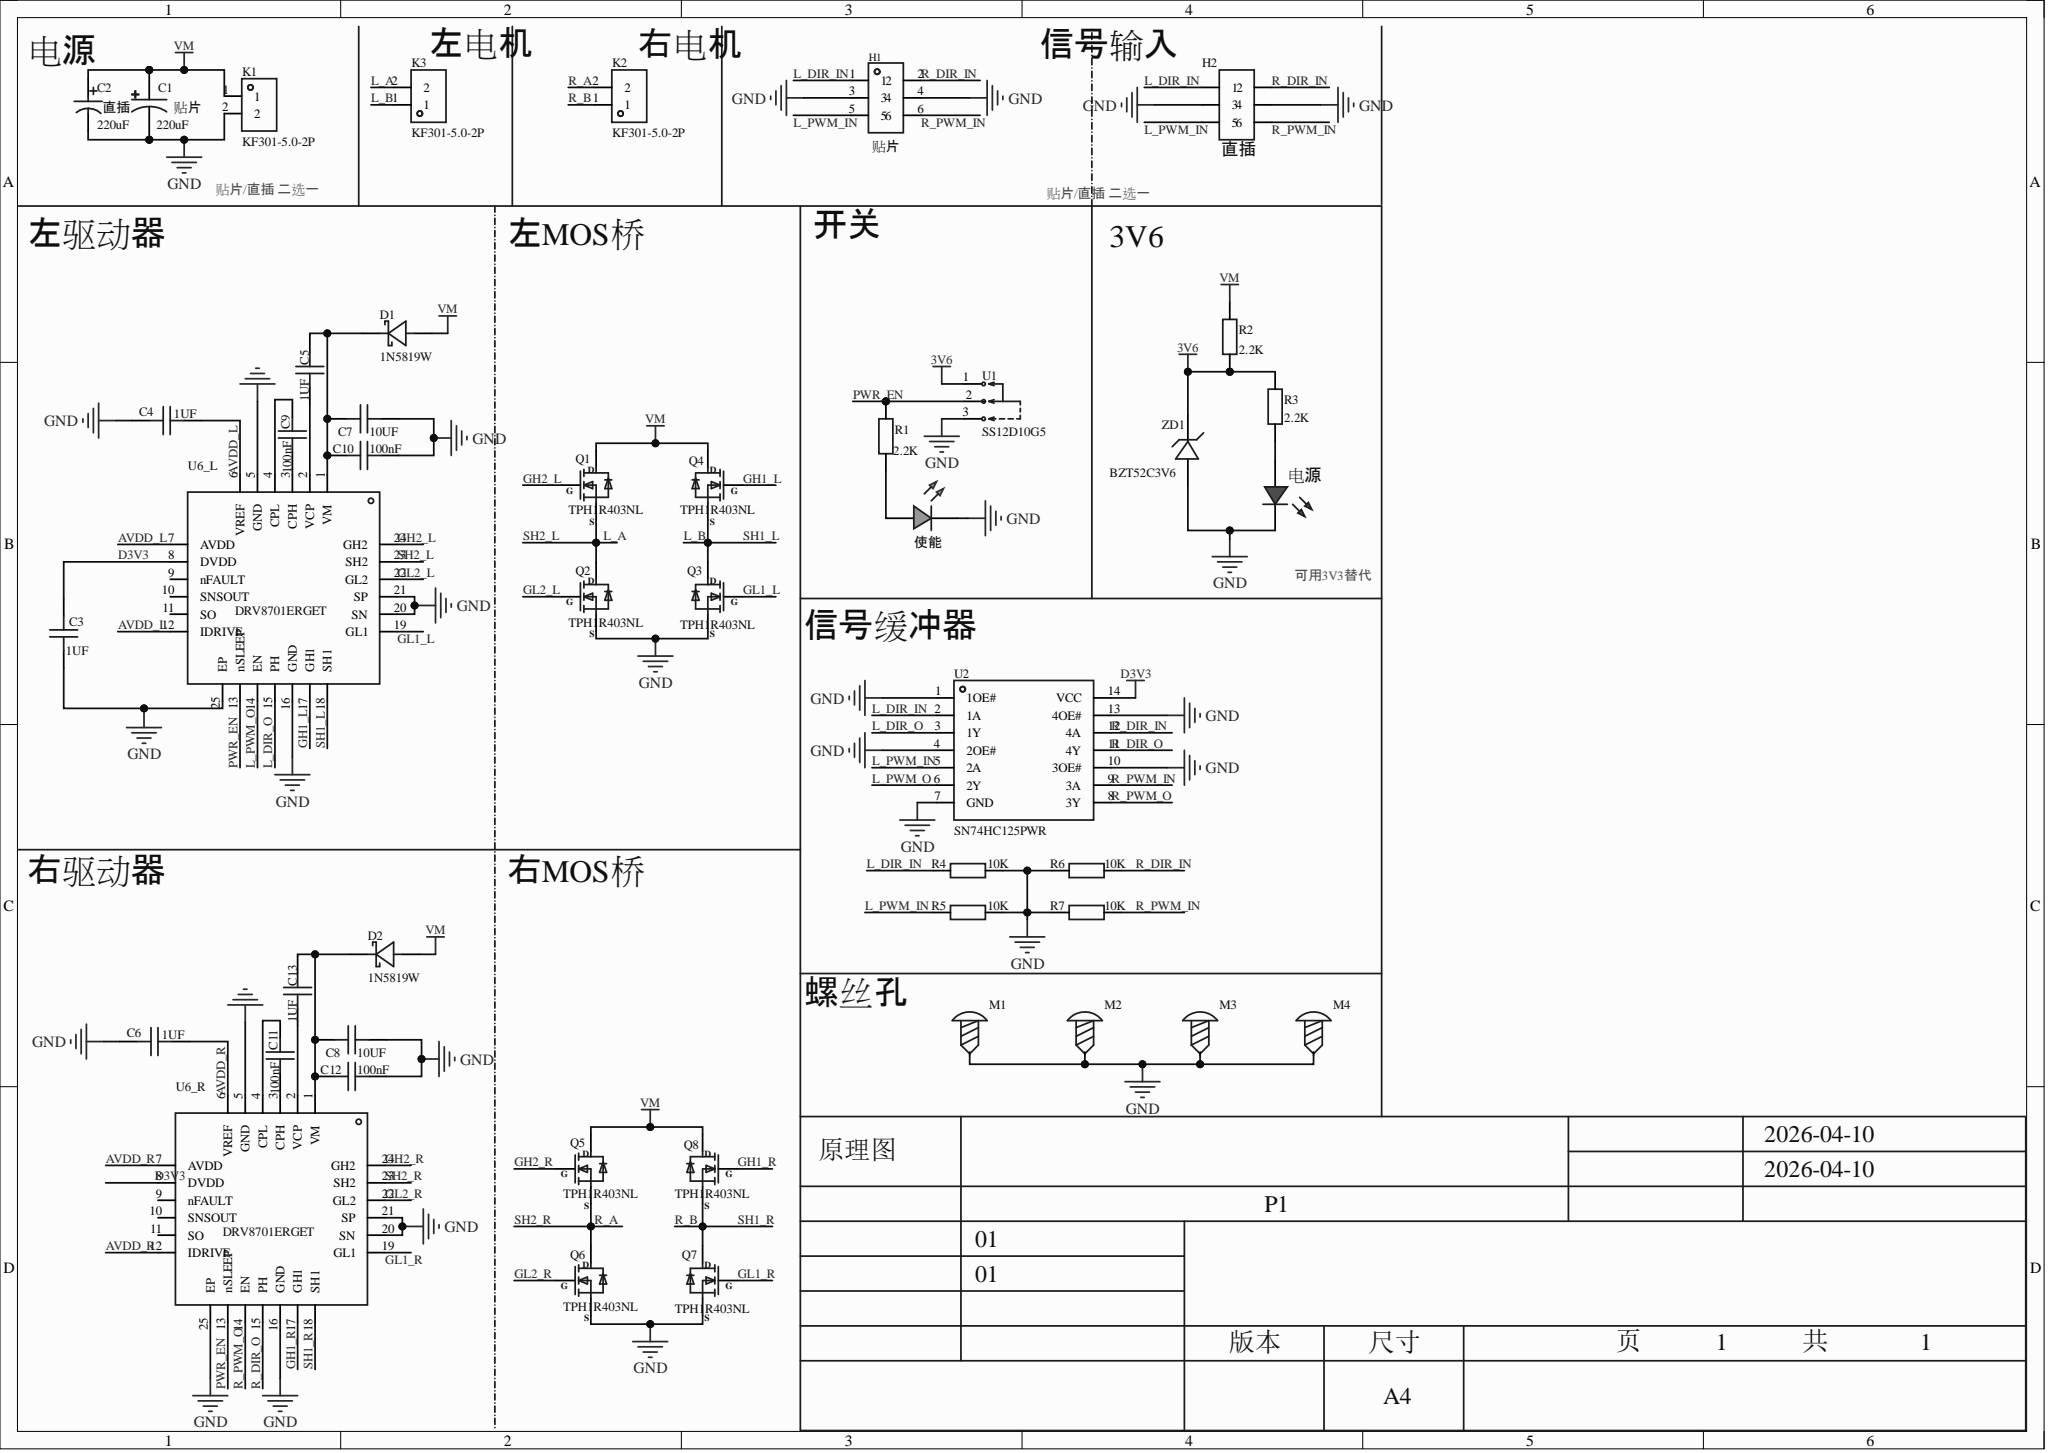Circuit board | Altium Designer | 46 parts | 37 nets
Bill of materials:
Comment,Description,Designator,Footprint,LibRef,Quantity
"220uF","","C1","CAP-SMD_BD8.0-L8.3-W8.3-FD","EEEFT1H221GP","1"
"220uF","容值:220uF;精度:±20%;额定电压:35V;","C2","CAP-TH_BD8.0-P3.50-D0.6-FD","ERS1VM221F12OT","1"
"1UF","","C3, C4, C5, C6, C13","C0603","CAP_0603","5"
"10UF","","C7, C8","C0603","CAP_0603","2"
"100nF","","C9, C10, C11, C12","C0603","CAP_0603","4"
"1N5819W","二极管配置:-;正向压降(Vf):900mV@3A;直流反向耐压(Vr):40V;平均整流电流(Io):1A;","D1, D2","SOD-123_L2.7-W1.6-LS3.7-RD-1","1N5819W","2"
"贴片","插针结构:-;间距:2.54mm;行距:-;圆针/方针:-;安装类型:-;排数:双排;总PIN位数:6P;额定电流:-;额定电压:-;配合针长度:-;塑高:-;触头材质:-;触头镀层:-;颜色:黑色;","H1","HDR-SMD_6P-P2.54-V-M-R2-C5-S7.4","2.54-2*3P立贴针","1"
"","","H2","HDR-TH_6P-P2.54-V-R2-C3-S2.54_A2541WV-2X3P","HDR-M_2.54_2x3","1"
"KF301-5.0-2P","结构:1x2P;间距:5mm;颜色:蓝色;安装方式:直插;额定电流:17A;额定电压:250V;排数:1;线规 - AWG:14~22;线规 - 平方毫米:1.5;每排PIN数:2;工作温度范围:-30℃~+120℃;","K1, K2, K3","CONN-TH_P5.00_KF301-5.0-2P","KF301-5.0-2P","3"
"","","M1, M2, M3, M4","M4螺丝","M4螺丝","4"
"TPH1R403NL","","Q1, Q2, Q3, Q4, Q5, Q6, Q7, Q8","DFN5x6","TPH1R403NL","8"
"2.2K","","R1, R2, R3","R0603","Res_0603","3"
"10K","","R4, R5, R6, R7","R0603","Res_0603","4"
"SS12D10G5","电路结构:单刀双掷;安装方式:直插;额定电流(DC):2A;额定电压(DC):125V;机械寿命:3千次;","U1","SW-TH_SHOU-HAN_SS12D10G4","SS12D10G5","1"
"SN74HC125PWR","输入类型:-;电源电压:2V~6V;元件数:4;每个元件位数:1;灌电流(IOL):7.8mA;拉电流(IOH):7.8mA;","U2","TSSOP-14_L5.0-W4.4-P0.65-LS6.5-BL","SN74HC125PWR","1"
"DRV8701ERGET","DRV8701 47V H 桥智能栅极驱动器","U6_L, U6_R","VQFN-24_L4.0-W4.0-P0.50-BL-EP2.5","DRV8701ERGET","2"
"BZT52C3V6","二极管配置:独立式;稳压值(标称值):3.6V;稳压值(范围):3.4V~3.8V;功率:350mW;精度:-;","ZD1","SOD-123_L2.8-W1.8-LS3.7-RD","BZT52C3V6_C2113","1"
"","","使能, 电源","LED_0603","LED_0603-G, LED_0603-R","2"
Netlist (Protel format):
[
C1
CAP-SMD_BD8.0-L8.3-W8.3-FD
220uF



]
[
C2
CAP-TH_BD8.0-P3.50-D0.6-FD
220uF



]
[
C3
C0603
1UF



]
[
C4
C0603
1UF



]
[
C5
C0603
1UF



]
[
C6
C0603
1UF



]
[
C7
C0603
10UF



]
[
C8
C0603
10UF



]
[
C9
C0603
100nF



]
[
C10
C0603
100nF



]
[
C11
C0603
100nF



]
[
C12
C0603
100nF



]
[
C13
C0603
1UF



]
[
D1
SOD-123_L2.7-W1.6-LS3.7-RD-1
1N5819W



]
[
D2
SOD-123_L2.7-W1.6-LS3.7-RD-1
1N5819W



]
[
H1
HDR-SMD_6P-P2.54-V-M-R2-C5-S7.4
贴片



]
[
H2
HDR-TH_6P-P2.54-V-R2-C3-S2.54_A2541WV-2X3P




]
[
K1
CONN-TH_P5.00_KF301-5.0-2P
KF301-5.0-2P



]
[
K2
CONN-TH_P5.00_KF301-5.0-2P
KF301-5.0-2P



]
[
K3
CONN-TH_P5.00_KF301-5.0-2P
KF301-5.0-2P



]
[
M1
M4螺丝




]
[
M2
M4螺丝




]
[
M3
M4螺丝




]
[
M4
M4螺丝




]
[
Q1
DFN5x6
TPH1R403NL



]
[
Q2
DFN5x6
TPH1R403NL



]
[
Q3
DFN5x6
TPH1R403NL



]
[
Q4
DFN5x6
TPH1R403NL



]
[
Q5
DFN5x6
TPH1R403NL



]
[
Q6
DFN5x6
TPH1R403NL



]
[
Q7
DFN5x6
TPH1R403NL



]
[
Q8
DFN5x6
TPH1R403NL



]
[
R1
R0603
2.2K



]
[
R2
R0603
2.2K



]
[
R3
R0603
2.2K



]
[
R4
R0603
10K



]
[
R5
R0603
10K



]
[
R6
R0603
10K



]
[
R7
R0603
10K



]
[
U1
SW-TH_SHOU-HAN_SS12D10G4
SS12D10G5



]
[
U2
TSSOP-14_L5.0-W4.4-P0.65-LS6.5-BL
SN74HC125PWR



]
[
U6_L
VQFN-24_L4.0-W4.0-P0.50-BL-EP2.5
DRV8701ERGET



]
[
U6_R
VQFN-24_L4.0-W4.0-P0.50-BL-EP2.5
DRV8701ERGET



]
[
ZD1
SOD-123_L2.8-W1.8-LS3.7-RD
BZT52C3V6



]
[
使能
LED_0603




]
[
电源
LED_0603




]
(
VM
C1-1
C2-1
D1-2
D2-2
K1-1
Q1-1
Q4-1
Q5-1
Q8-1
R2-2
)
(
R_PWM_O
U2-8
U6_R-14
)
(
R_PWM_IN
H1-6
H2-6
R7-2
U2-9
)
(
R_DIR_O
U2-11
U6_R-15
)
(
R_DIR_IN
H1-2
H2-2
R6-2
U2-12
)
(
R_B
K2-1
Q7-1
Q8-3
U6_R-18
)
(
R_A
K2-2
Q5-3
Q6-1
U6_R-23
)
(
PWR_EN
R1-2
U1-2
U6_L-13
U6_R-13
)
(
NetR3_1
R3-1
电源-2
)
(
NetR1_1
R1-1
使能-2
)
(
NetC13_2
C13-2
U6_R-2
)
(
NetC11_2
C11-2
U6_R-4
)
(
NetC11_1
C11-1
U6_R-3
)
(
NetC9_2
C9-2
U6_L-4
)
(
NetC9_1
C9-1
U6_L-3
)
(
NetC8_1
C8-1
C12-1
C13-1
D2-1
U6_R-1
)
(
NetC5_2
C5-2
U6_L-2
)
(
NetC5_1
C5-1
C7-1
C10-1
D1-1
U6_L-1
)
(
L_PWM_O
U2-6
U6_L-14
)
(
L_PWM_IN
H1-5
H2-5
R5-1
U2-5
)
(
L_DIR_O
U2-3
U6_L-15
)
(
L_DIR_IN
H1-1
H2-1
R4-1
U2-2
)
(
L_B
K3-1
Q3-1
Q4-3
U6_L-18
)
(
L_A
K3-2
Q1-3
Q2-1
U6_L-23
)
(
GND
C1-2
C2-2
C3-1
C4-2
C6-2
C7-2
C8-2
C10-2
C12-2
H1-3
H1-4
H2-3
H2-4
K1-2
M1-1
M2-1
M3-1
M4-1
Q2-3
Q3-3
Q6-3
Q7-3
R4-2
R5-2
R6-1
R7-1
U1-3
U2-1
U2-4
U2-7
U2-10
U2-13
U6_L-5
U6_L-16
U6_L-20
U6_L-21
U6_L-25
U6_R-5
U6_R-16
U6_R-20
U6_R-21
U6_R-25
ZD1-2
使能-1
电源-1
)
(
GL2_R
Q6-2
U6_R-22
)
(
GL2_L
Q2-2
U6_L-22
)
(
GL1_R
Q7-2
U6_R-19
)
(
GL1_L
Q3-2
U6_L-19
)
(
GH2_R
Q5-2
U6_R-24
)
(
GH2_L
Q1-2
U6_L-24
)
(
GH1_R
Q8-2
U6_R-17
)
(
GH1_L
Q4-2
U6_L-17
)
(
D3V3
C3-2
U2-14
U6_L-8
U6_R-8
)
(
AVDD_R
C6-1
U6_R-6
U6_R-7
U6_R-12
)
(
AVDD_L
C4-1
U6_L-6
U6_L-7
U6_L-12
)
(
3V6
R2-1
R3-2
U1-1
ZD1-1
)